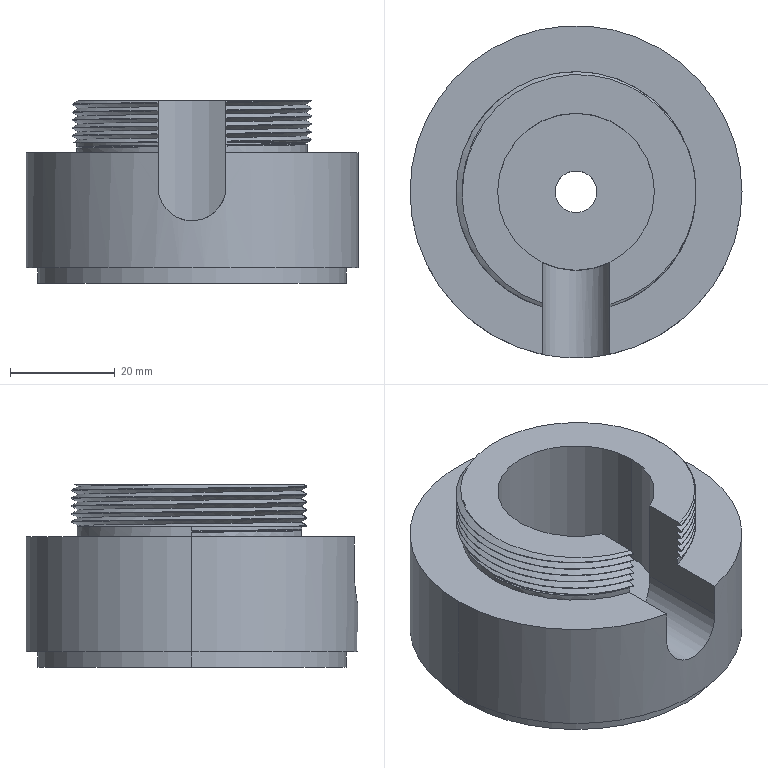Part | STEP file | output terminal^spray gun PTFE model | 1 solid | 69 faces | box 63.5 x 63.5 x 35 mm | volume 72808 mm3 | cylinder 38 | spline 15 | plane 10 | cone 6 | commonest cylinder face diameters 45.9 x17 3.3 x6 44 x5 30 x3 8 x2 59 x2